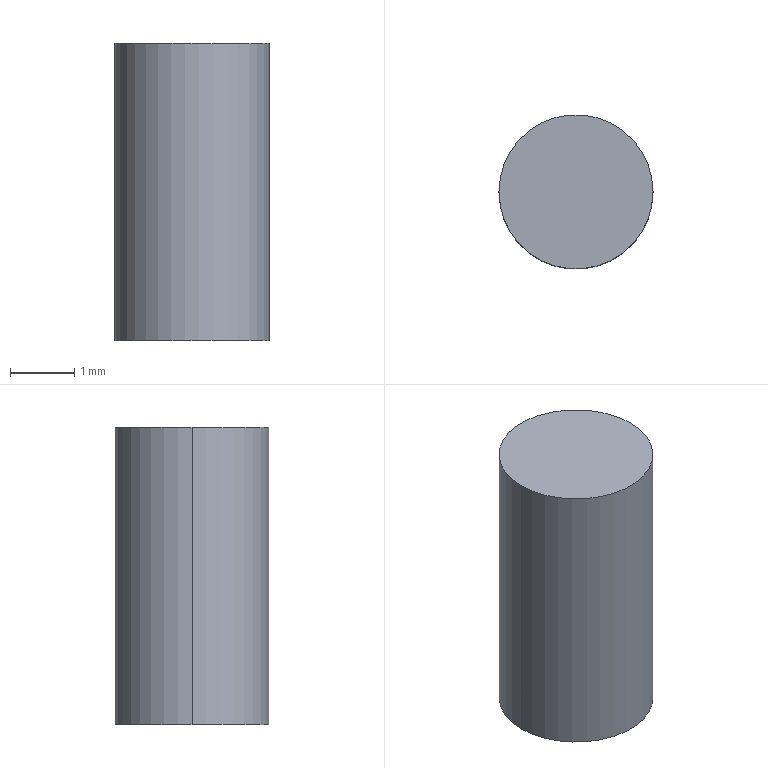Part | SolidWorks | features BaseBody 1 | 1 solid | 4 faces | box 2.4 x 2.4 x 4.64 mm | volume 20.991 mm3 | cylinder 2 | plane 2 | commonest cylinder face diameters 2.4 x2
STEP:
#1=CARTESIAN_POINT('',(567.42,76.38,42.313));
#2=VERTEX_POINT('',#1);
#3=CARTESIAN_POINT('',(565.02,76.38,42.313));
#4=VERTEX_POINT('',#3);
#5=CARTESIAN_POINT('',(566.22,76.38,42.313));
#6=DIRECTION('',(0.,0.,1.));
#7=DIRECTION('',(1.,0.,0.));
#8=AXIS2_PLACEMENT_3D('',#5,#6,#7);
#9=CIRCLE('',#8,1.2);
#10=EDGE_CURVE('',#2,#4,#9,.T.);
#11=ORIENTED_EDGE('',*,*,#10,.T.);
#12=CARTESIAN_POINT('',(565.02,76.38,46.953));
#13=VERTEX_POINT('',#12);
#14=CARTESIAN_POINT('',(565.02,76.38,44.633));
#15=DIRECTION('',(0.,0.,1.));
#16=VECTOR('',#15,1000.);
#17=LINE('',#14,#16);
#18=EDGE_CURVE('',#4,#13,#17,.T.);
#19=ORIENTED_EDGE('',*,*,#18,.T.);
#20=CARTESIAN_POINT('',(567.42,76.38,46.953));
#21=VERTEX_POINT('',#20);
#22=CARTESIAN_POINT('',(566.22,76.38,46.953));
#23=DIRECTION('',(0.,0.,-1.));
#24=DIRECTION('',(1.,0.,0.));
#25=AXIS2_PLACEMENT_3D('',#22,#23,#24);
#26=CIRCLE('',#25,1.2);
#27=EDGE_CURVE('',#13,#21,#26,.T.);
#28=ORIENTED_EDGE('',*,*,#27,.T.);
#29=CARTESIAN_POINT('',(567.42,76.38,44.633));
#30=DIRECTION('',(0.,0.,1.));
#31=VECTOR('',#30,1000.);
#32=LINE('',#29,#31);
#33=EDGE_CURVE('',#2,#21,#32,.T.);
#34=ORIENTED_EDGE('',*,*,#33,.F.);
#35=EDGE_LOOP('',(#11,#19,#28,#34));
#36=FACE_OUTER_BOUND('',#35,.T.);
#37=CARTESIAN_POINT('',(566.22,76.38,44.633));
#38=DIRECTION('',(0.,0.,1.));
#39=DIRECTION('',(1.,0.,0.));
#40=AXIS2_PLACEMENT_3D('',#37,#38,#39);
#41=CYLINDRICAL_SURFACE('',#40,1.2);
#42=ADVANCED_FACE('',(#36),#41,.T.);
#43=ORIENTED_EDGE('',*,*,#18,.F.);
#44=CARTESIAN_POINT('',(566.22,76.38,42.313));
#45=DIRECTION('',(0.,0.,1.));
#46=DIRECTION('',(1.,0.,0.));
#47=AXIS2_PLACEMENT_3D('',#44,#45,#46);
#48=CIRCLE('',#47,1.2);
#49=EDGE_CURVE('',#4,#2,#48,.T.);
#50=ORIENTED_EDGE('',*,*,#49,.T.);
#51=ORIENTED_EDGE('',*,*,#33,.T.);
#52=CARTESIAN_POINT('',(566.22,76.38,46.953));
#53=DIRECTION('',(0.,0.,-1.));
#54=DIRECTION('',(1.,0.,0.));
#55=AXIS2_PLACEMENT_3D('',#52,#53,#54);
#56=CIRCLE('',#55,1.2);
#57=EDGE_CURVE('',#21,#13,#56,.T.);
#58=ORIENTED_EDGE('',*,*,#57,.T.);
#59=EDGE_LOOP('',(#43,#50,#51,#58));
#60=FACE_OUTER_BOUND('',#59,.T.);
#61=CARTESIAN_POINT('',(566.22,76.38,44.633));
#62=DIRECTION('',(0.,0.,1.));
#63=DIRECTION('',(1.,0.,0.));
#64=AXIS2_PLACEMENT_3D('',#61,#62,#63);
#65=CYLINDRICAL_SURFACE('',#64,1.2);
#66=ADVANCED_FACE('',(#60),#65,.T.);
#67=ORIENTED_EDGE('',*,*,#57,.F.);
#68=ORIENTED_EDGE('',*,*,#27,.F.);
#69=EDGE_LOOP('',(#67,#68));
#70=FACE_OUTER_BOUND('',#69,.T.);
#71=CARTESIAN_POINT('',(566.493,76.38,46.953));
#72=DIRECTION('',(0.,0.,-1.));
#73=DIRECTION('',(-1.,0.,0.));
#74=AXIS2_PLACEMENT_3D('',#71,#72,#73);
#75=PLANE('',#74);
#76=ADVANCED_FACE('',(#70),#75,.F.);
#77=ORIENTED_EDGE('',*,*,#10,.F.);
#78=ORIENTED_EDGE('',*,*,#49,.F.);
#79=EDGE_LOOP('',(#77,#78));
#80=FACE_OUTER_BOUND('',#79,.T.);
#81=CARTESIAN_POINT('',(565.99,76.934,42.313));
#82=DIRECTION('',(0.,0.,1.));
#83=DIRECTION('',(1.,0.,0.));
#84=AXIS2_PLACEMENT_3D('',#81,#82,#83);
#85=PLANE('',#84);
#86=ADVANCED_FACE('',(#80),#85,.F.);
#87=CLOSED_SHELL('',(#42,#66,#76,#86));
#88=MANIFOLD_SOLID_BREP('',#87);
#89=CARTESIAN_POINT('',(0.,0.,0.));
#90=DIRECTION('',(0.,0.,1.));
#91=DIRECTION('',(1.,0.,0.));
#92=AXIS2_PLACEMENT_3D('',#89,#90,#91);
#93=(LENGTH_UNIT()NAMED_UNIT(*)SI_UNIT(.MILLI.,.METRE.));
#94=UNCERTAINTY_MEASURE_WITH_UNIT(LENGTH_MEASURE(0.00001),#93,'','');
#95=(NAMED_UNIT(*)PLANE_ANGLE_UNIT()SI_UNIT($,.RADIAN.));
#96=(NAMED_UNIT(*)SI_UNIT($,.STERADIAN.)SOLID_ANGLE_UNIT());
#97=(GEOMETRIC_REPRESENTATION_CONTEXT(3)GLOBAL_UNCERTAINTY_ASSIGNED_CONTEXT((#94))GLOBAL_UNIT_ASSIGNED_CONTEXT((#93,#95,#96))REPRESENTATION_CONTEXT('',''));
#98=ADVANCED_BREP_SHAPE_REPRESENTATION('',(#88,#92),#97);